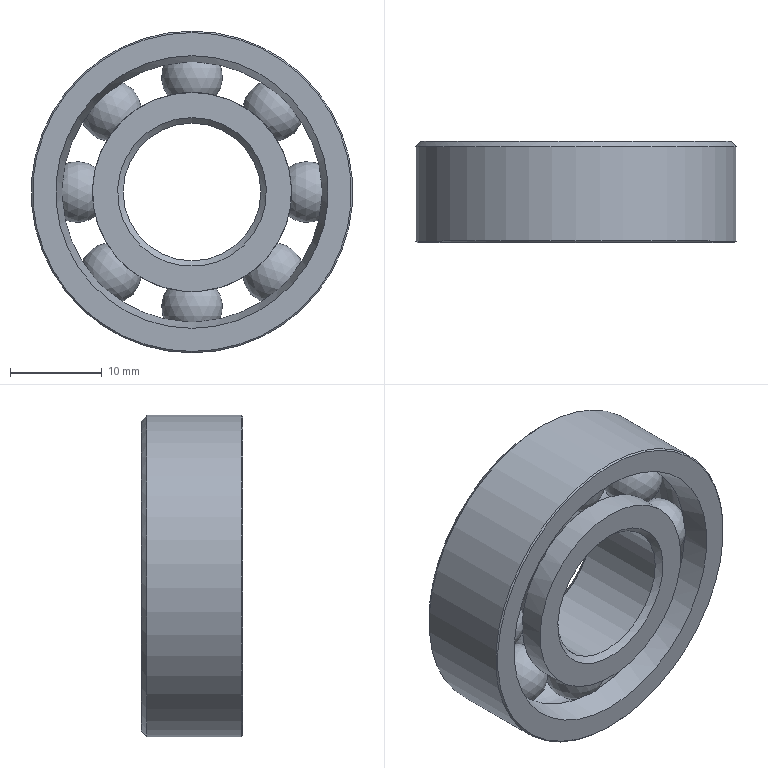Part | STEP file | YBQDJ-PD-20 | 1 solid | 38 faces | box 35 x 11 x 35 mm | volume 5907 mm3 | torus 16 | sphere 8 | cylinder 5 | cone 5 | plane 4 | commonest cylinder face diameters 21.667 x2 15 x1 28.333 x1 35 x1